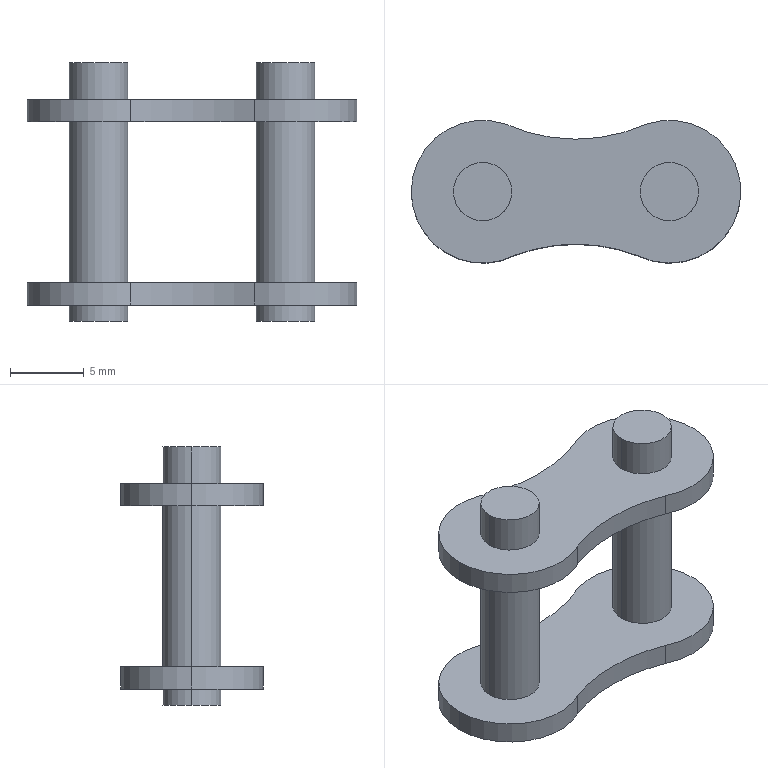Part | STEP file | CHEL40Achain-3 | 1 solid | 30 faces | box 22.4 x 9.7 x 17.55 mm | volume 895.476 mm3 | cylinder 22 | plane 8 | commonest cylinder face diameters 3.97 x12 9.7 x6 23.4 x4